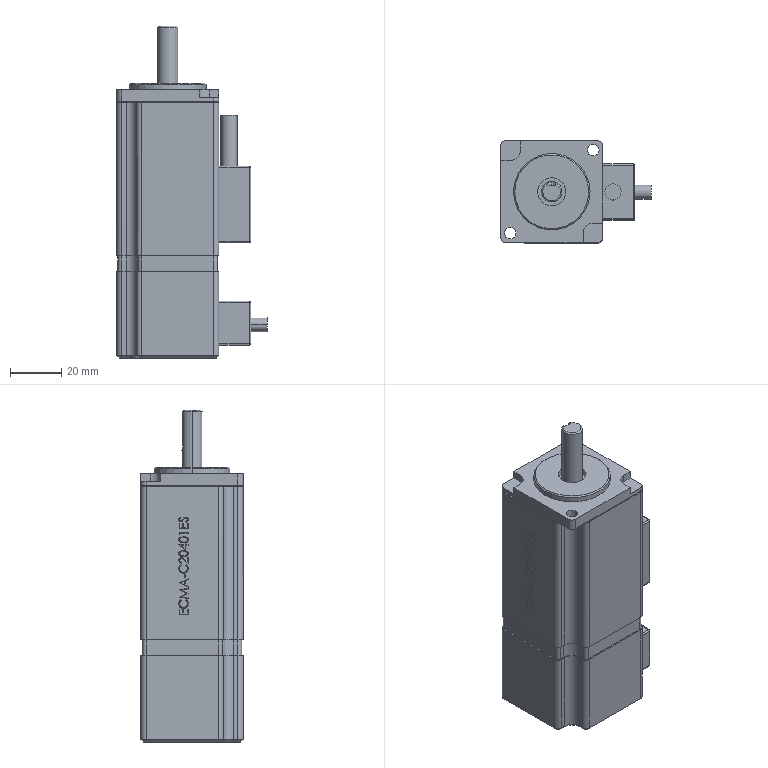Part | STEP file | 100W servo motor (100W Delta servo motor) | 1 solid | 334 faces | box 59 x 40 x 130.1 mm | volume 171789 mm3 | plane 184 | cylinder 68 | spline 57 | cone 17 | sphere 8 | commonest cylinder face diameters 4 x20 1 x16 8 x10 3 x8 4.5 x4 5.5 x2